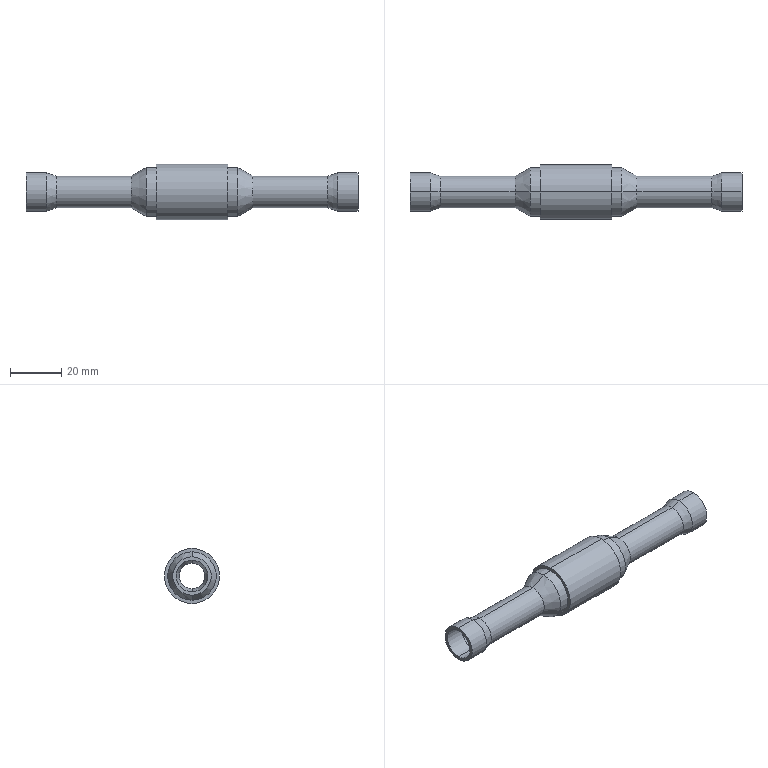Part | STEP file | stop valve | 1 solid | 50 faces | box 130 x 21.6 x 21.6 mm | volume 7854 mm3 | cylinder 28 | cone 16 | plane 6 | commonest cylinder face diameters 19 x6 9.9 x4 12.4 x4 12.5 x4 15 x4 16.4 x4